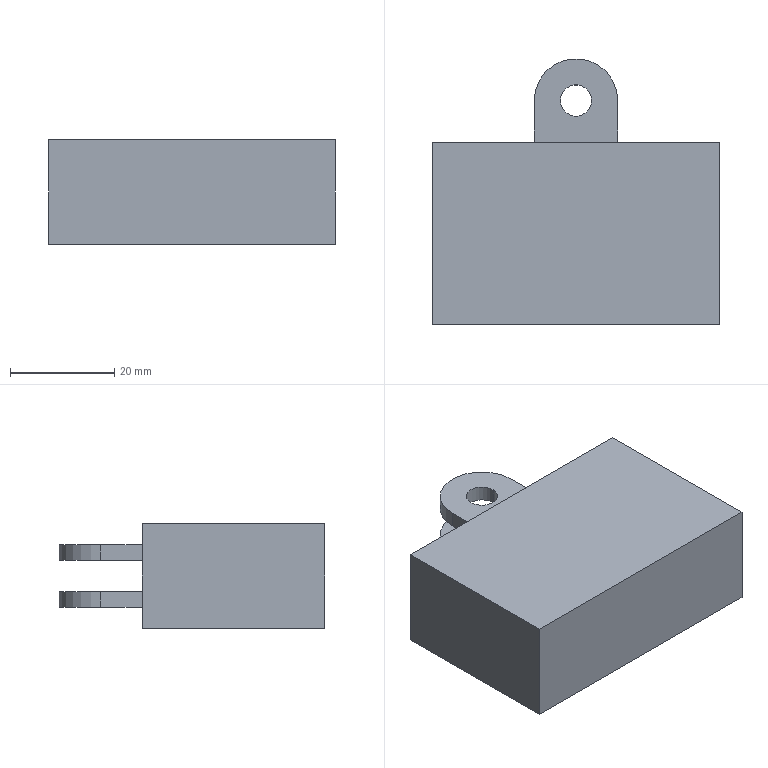Part | SolidWorks | features ICE 3, Extrusion 1 | 1 solid | 20 faces | box 55 x 51 x 20 mm | volume 39702 mm3 | plane 14 | cylinder 6 | commonest cylinder face diameters 6 x4 16 x2
STEP:
#1=CARTESIAN_POINT('',(-3.,25.5,4.));
#2=VERTEX_POINT('',#1);
#3=CARTESIAN_POINT('',(3.,25.5,4.));
#4=VERTEX_POINT('',#3);
#5=CARTESIAN_POINT('',(0.,25.5,4.));
#6=DIRECTION('',(0.,0.,1.));
#7=DIRECTION('',(1.,0.,0.));
#8=AXIS2_PLACEMENT_3D('',#5,#6,#7);
#9=CIRCLE('',#8,3.);
#10=EDGE_CURVE('',#2,#4,#9,.T.);
#11=ORIENTED_EDGE('',*,*,#10,.F.);
#12=CARTESIAN_POINT('',(-3.,25.5,7.));
#13=VERTEX_POINT('',#12);
#14=CARTESIAN_POINT('',(-3.,25.5,0.));
#15=DIRECTION('',(0.,0.,1.));
#16=VECTOR('',#15,1000.);
#17=LINE('',#14,#16);
#18=EDGE_CURVE('',#2,#13,#17,.T.);
#19=ORIENTED_EDGE('',*,*,#18,.T.);
#20=CARTESIAN_POINT('',(3.,25.5,7.));
#21=VERTEX_POINT('',#20);
#22=CARTESIAN_POINT('',(0.,25.5,7.));
#23=DIRECTION('',(0.,0.,1.));
#24=DIRECTION('',(1.,0.,0.));
#25=AXIS2_PLACEMENT_3D('',#22,#23,#24);
#26=CIRCLE('',#25,3.);
#27=EDGE_CURVE('',#13,#21,#26,.T.);
#28=ORIENTED_EDGE('',*,*,#27,.T.);
#29=CARTESIAN_POINT('',(3.,25.5,0.));
#30=DIRECTION('',(0.,0.,1.));
#31=VECTOR('',#30,1000.);
#32=LINE('',#29,#31);
#33=EDGE_CURVE('',#4,#21,#32,.T.);
#34=ORIENTED_EDGE('',*,*,#33,.F.);
#35=EDGE_LOOP('',(#11,#19,#28,#34));
#36=FACE_OUTER_BOUND('',#35,.T.);
#37=CARTESIAN_POINT('',(0.,25.5,0.));
#38=DIRECTION('',(0.,0.,1.));
#39=DIRECTION('',(1.,0.,0.));
#40=AXIS2_PLACEMENT_3D('',#37,#38,#39);
#41=CYLINDRICAL_SURFACE('',#40,3.);
#42=ADVANCED_FACE('',(#36),#41,.F.);
#43=CARTESIAN_POINT('',(3.,25.5,13.));
#44=VERTEX_POINT('',#43);
#45=CARTESIAN_POINT('',(-3.,25.5,13.));
#46=VERTEX_POINT('',#45);
#47=CARTESIAN_POINT('',(0.,25.5,13.));
#48=DIRECTION('',(0.,0.,-1.));
#49=DIRECTION('',(-1.,0.,0.));
#50=AXIS2_PLACEMENT_3D('',#47,#48,#49);
#51=CIRCLE('',#50,3.);
#52=EDGE_CURVE('',#44,#46,#51,.T.);
#53=ORIENTED_EDGE('',*,*,#52,.T.);
#54=CARTESIAN_POINT('',(-3.,25.5,16.));
#55=VERTEX_POINT('',#54);
#56=CARTESIAN_POINT('',(-3.,25.5,0.));
#57=DIRECTION('',(0.,0.,1.));
#58=VECTOR('',#57,1000.);
#59=LINE('',#56,#58);
#60=EDGE_CURVE('',#46,#55,#59,.T.);
#61=ORIENTED_EDGE('',*,*,#60,.T.);
#62=CARTESIAN_POINT('',(3.,25.5,16.));
#63=VERTEX_POINT('',#62);
#64=CARTESIAN_POINT('',(0.,25.5,16.));
#65=DIRECTION('',(0.,0.,1.));
#66=DIRECTION('',(1.,0.,0.));
#67=AXIS2_PLACEMENT_3D('',#64,#65,#66);
#68=CIRCLE('',#67,3.);
#69=EDGE_CURVE('',#55,#63,#68,.T.);
#70=ORIENTED_EDGE('',*,*,#69,.T.);
#71=CARTESIAN_POINT('',(3.,25.5,0.));
#72=DIRECTION('',(0.,0.,1.));
#73=VECTOR('',#72,1000.);
#74=LINE('',#71,#73);
#75=EDGE_CURVE('',#44,#63,#74,.T.);
#76=ORIENTED_EDGE('',*,*,#75,.F.);
#77=EDGE_LOOP('',(#53,#61,#70,#76));
#78=FACE_OUTER_BOUND('',#77,.T.);
#79=CARTESIAN_POINT('',(0.,25.5,0.));
#80=DIRECTION('',(0.,0.,1.));
#81=DIRECTION('',(1.,0.,0.));
#82=AXIS2_PLACEMENT_3D('',#79,#80,#81);
#83=CYLINDRICAL_SURFACE('',#82,3.);
#84=ADVANCED_FACE('',(#78),#83,.F.);
#85=CARTESIAN_POINT('',(-8.,25.5,4.));
#86=VERTEX_POINT('',#85);
#87=CARTESIAN_POINT('',(-8.,17.5,4.));
#88=VERTEX_POINT('',#87);
#89=CARTESIAN_POINT('',(-8.,33.5,4.));
#90=DIRECTION('',(0.,-1.,0.));
#91=VECTOR('',#90,1000.);
#92=LINE('',#89,#91);
#93=EDGE_CURVE('',#86,#88,#92,.T.);
#94=ORIENTED_EDGE('',*,*,#93,.F.);
#95=CARTESIAN_POINT('',(8.,25.5,4.));
#96=VERTEX_POINT('',#95);
#97=CARTESIAN_POINT('',(0.,25.5,4.));
#98=DIRECTION('',(0.,0.,-1.));
#99=DIRECTION('',(1.,0.,0.));
#100=AXIS2_PLACEMENT_3D('',#97,#98,#99);
#101=CIRCLE('',#100,8.);
#102=EDGE_CURVE('',#86,#96,#101,.T.);
#103=ORIENTED_EDGE('',*,*,#102,.T.);
#104=CARTESIAN_POINT('',(8.,17.5,4.));
#105=VERTEX_POINT('',#104);
#106=CARTESIAN_POINT('',(8.,33.5,4.));
#107=DIRECTION('',(0.,-1.,0.));
#108=VECTOR('',#107,1000.);
#109=LINE('',#106,#108);
#110=EDGE_CURVE('',#96,#105,#109,.T.);
#111=ORIENTED_EDGE('',*,*,#110,.T.);
#112=CARTESIAN_POINT('',(-8.,17.5,4.));
#113=DIRECTION('',(-1.,0.,0.));
#114=VECTOR('',#113,1000.);
#115=LINE('',#112,#114);
#116=EDGE_CURVE('',#105,#88,#115,.T.);
#117=ORIENTED_EDGE('',*,*,#116,.T.);
#118=EDGE_LOOP('',(#94,#103,#111,#117));
#119=FACE_OUTER_BOUND('',#118,.T.);
#120=CARTESIAN_POINT('',(0.,25.5,4.));
#121=DIRECTION('',(0.,0.,1.));
#122=DIRECTION('',(1.,0.,0.));
#123=AXIS2_PLACEMENT_3D('',#120,#121,#122);
#124=CIRCLE('',#123,3.);
#125=EDGE_CURVE('',#4,#2,#124,.T.);
#126=ORIENTED_EDGE('',*,*,#125,.T.);
#127=ORIENTED_EDGE('',*,*,#10,.T.);
#128=EDGE_LOOP('',(#126,#127));
#129=FACE_BOUND('',#128,.T.);
#130=CARTESIAN_POINT('',(-8.,33.5,4.));
#131=DIRECTION('',(0.,0.,1.));
#132=DIRECTION('',(1.,0.,0.));
#133=AXIS2_PLACEMENT_3D('',#130,#131,#132);
#134=PLANE('',#133);
#135=ADVANCED_FACE('',(#119,#129),#134,.F.);
#136=CARTESIAN_POINT('',(8.,25.5,16.));
#137=VERTEX_POINT('',#136);
#138=CARTESIAN_POINT('',(8.,17.5,16.));
#139=VERTEX_POINT('',#138);
#140=CARTESIAN_POINT('',(8.,33.5,16.));
#141=DIRECTION('',(0.,-1.,0.));
#142=VECTOR('',#141,1000.);
#143=LINE('',#140,#142);
#144=EDGE_CURVE('',#137,#139,#143,.T.);
#145=ORIENTED_EDGE('',*,*,#144,.F.);
#146=CARTESIAN_POINT('',(-8.,25.5,16.));
#147=VERTEX_POINT('',#146);
#148=CARTESIAN_POINT('',(0.,25.5,16.));
#149=DIRECTION('',(0.,0.,-1.));
#150=DIRECTION('',(1.,0.,0.));
#151=AXIS2_PLACEMENT_3D('',#148,#149,#150);
#152=CIRCLE('',#151,8.);
#153=EDGE_CURVE('',#147,#137,#152,.T.);
#154=ORIENTED_EDGE('',*,*,#153,.F.);
#155=CARTESIAN_POINT('',(-8.,17.5,16.));
#156=VERTEX_POINT('',#155);
#157=CARTESIAN_POINT('',(-8.,33.5,16.));
#158=DIRECTION('',(0.,-1.,0.));
#159=VECTOR('',#158,1000.);
#160=LINE('',#157,#159);
#161=EDGE_CURVE('',#147,#156,#160,.T.);
#162=ORIENTED_EDGE('',*,*,#161,.T.);
#163=CARTESIAN_POINT('',(-8.,17.5,16.));
#164=DIRECTION('',(1.,0.,0.));
#165=VECTOR('',#164,1000.);
#166=LINE('',#163,#165);
#167=EDGE_CURVE('',#156,#139,#166,.T.);
#168=ORIENTED_EDGE('',*,*,#167,.T.);
#169=EDGE_LOOP('',(#145,#154,#162,#168));
#170=FACE_OUTER_BOUND('',#169,.T.);
#171=CARTESIAN_POINT('',(0.,25.5,16.));
#172=DIRECTION('',(0.,0.,1.));
#173=DIRECTION('',(1.,0.,0.));
#174=AXIS2_PLACEMENT_3D('',#171,#172,#173);
#175=CIRCLE('',#174,3.);
#176=EDGE_CURVE('',#63,#55,#175,.T.);
#177=ORIENTED_EDGE('',*,*,#176,.F.);
#178=ORIENTED_EDGE('',*,*,#69,.F.);
#179=EDGE_LOOP('',(#177,#178));
#180=FACE_BOUND('',#179,.T.);
#181=CARTESIAN_POINT('',(-8.,33.5,16.));
#182=DIRECTION('',(0.,0.,-1.));
#183=DIRECTION('',(-1.,0.,0.));
#184=AXIS2_PLACEMENT_3D('',#181,#182,#183);
#185=PLANE('',#184);
#186=ADVANCED_FACE('',(#170,#180),#185,.F.);
#187=CARTESIAN_POINT('',(-8.,25.5,7.));
#188=VERTEX_POINT('',#187);
#189=CARTESIAN_POINT('',(8.,25.5,7.));
#190=VERTEX_POINT('',#189);
#191=CARTESIAN_POINT('',(0.,25.5,7.));
#192=DIRECTION('',(0.,0.,-1.));
#193=DIRECTION('',(1.,0.,0.));
#194=AXIS2_PLACEMENT_3D('',#191,#192,#193);
#195=CIRCLE('',#194,8.);
#196=EDGE_CURVE('',#188,#190,#195,.T.);
#197=ORIENTED_EDGE('',*,*,#196,.F.);
#198=CARTESIAN_POINT('',(-8.,17.5,7.));
#199=VERTEX_POINT('',#198);
#200=CARTESIAN_POINT('',(-8.,33.5,7.));
#201=DIRECTION('',(0.,-1.,0.));
#202=VECTOR('',#201,1000.);
#203=LINE('',#200,#202);
#204=EDGE_CURVE('',#188,#199,#203,.T.);
#205=ORIENTED_EDGE('',*,*,#204,.T.);
#206=CARTESIAN_POINT('',(8.,17.5,7.));
#207=VERTEX_POINT('',#206);
#208=CARTESIAN_POINT('',(-8.,17.5,7.));
#209=DIRECTION('',(-1.,0.,0.));
#210=VECTOR('',#209,1000.);
#211=LINE('',#208,#210);
#212=EDGE_CURVE('',#207,#199,#211,.T.);
#213=ORIENTED_EDGE('',*,*,#212,.F.);
#214=CARTESIAN_POINT('',(8.,33.5,7.));
#215=DIRECTION('',(0.,-1.,0.));
#216=VECTOR('',#215,1000.);
#217=LINE('',#214,#216);
#218=EDGE_CURVE('',#190,#207,#217,.T.);
#219=ORIENTED_EDGE('',*,*,#218,.F.);
#220=EDGE_LOOP('',(#197,#205,#213,#219));
#221=FACE_OUTER_BOUND('',#220,.T.);
#222=CARTESIAN_POINT('',(0.,25.5,7.));
#223=DIRECTION('',(0.,0.,1.));
#224=DIRECTION('',(1.,0.,0.));
#225=AXIS2_PLACEMENT_3D('',#222,#223,#224);
#226=CIRCLE('',#225,3.);
#227=EDGE_CURVE('',#21,#13,#226,.T.);
#228=ORIENTED_EDGE('',*,*,#227,.F.);
#229=ORIENTED_EDGE('',*,*,#27,.F.);
#230=EDGE_LOOP('',(#228,#229));
#231=FACE_BOUND('',#230,.T.);
#232=CARTESIAN_POINT('',(-8.,33.5,7.));
#233=DIRECTION('',(0.,0.,1.));
#234=DIRECTION('',(1.,0.,0.));
#235=AXIS2_PLACEMENT_3D('',#232,#233,#234);
#236=PLANE('',#235);
#237=ADVANCED_FACE('',(#221,#231),#236,.T.);
#238=CARTESIAN_POINT('',(8.,25.5,13.));
#239=VERTEX_POINT('',#238);
#240=CARTESIAN_POINT('',(-8.,25.5,13.));
#241=VERTEX_POINT('',#240);
#242=CARTESIAN_POINT('',(0.,25.5,13.));
#243=DIRECTION('',(0.,0.,1.));
#244=DIRECTION('',(-1.,0.,0.));
#245=AXIS2_PLACEMENT_3D('',#242,#243,#244);
#246=CIRCLE('',#245,8.);
#247=EDGE_CURVE('',#239,#241,#246,.T.);
#248=ORIENTED_EDGE('',*,*,#247,.F.);
#249=CARTESIAN_POINT('',(8.,17.5,13.));
#250=VERTEX_POINT('',#249);
#251=CARTESIAN_POINT('',(8.,33.5,13.));
#252=DIRECTION('',(0.,-1.,0.));
#253=VECTOR('',#252,1000.);
#254=LINE('',#251,#253);
#255=EDGE_CURVE('',#239,#250,#254,.T.);
#256=ORIENTED_EDGE('',*,*,#255,.T.);
#257=CARTESIAN_POINT('',(-8.,17.5,13.));
#258=VERTEX_POINT('',#257);
#259=CARTESIAN_POINT('',(-8.,17.5,13.));
#260=DIRECTION('',(1.,0.,0.));
#261=VECTOR('',#260,1000.);
#262=LINE('',#259,#261);
#263=EDGE_CURVE('',#258,#250,#262,.T.);
#264=ORIENTED_EDGE('',*,*,#263,.F.);
#265=CARTESIAN_POINT('',(-8.,33.5,13.));
#266=DIRECTION('',(0.,-1.,0.));
#267=VECTOR('',#266,1000.);
#268=LINE('',#265,#267);
#269=EDGE_CURVE('',#241,#258,#268,.T.);
#270=ORIENTED_EDGE('',*,*,#269,.F.);
#271=EDGE_LOOP('',(#248,#256,#264,#270));
#272=FACE_OUTER_BOUND('',#271,.T.);
#273=ORIENTED_EDGE('',*,*,#52,.F.);
#274=CARTESIAN_POINT('',(0.,25.5,13.));
#275=DIRECTION('',(0.,0.,-1.));
#276=DIRECTION('',(-1.,0.,0.));
#277=AXIS2_PLACEMENT_3D('',#274,#275,#276);
#278=CIRCLE('',#277,3.);
#279=EDGE_CURVE('',#46,#44,#278,.T.);
#280=ORIENTED_EDGE('',*,*,#279,.F.);
#281=EDGE_LOOP('',(#273,#280));
#282=FACE_BOUND('',#281,.T.);
#283=CARTESIAN_POINT('',(-8.,33.5,13.));
#284=DIRECTION('',(0.,0.,-1.));
#285=DIRECTION('',(-1.,0.,0.));
#286=AXIS2_PLACEMENT_3D('',#283,#284,#285);
#287=PLANE('',#286);
#288=ADVANCED_FACE('',(#272,#282),#287,.T.);
#289=ORIENTED_EDGE('',*,*,#110,.F.);
#290=CARTESIAN_POINT('',(8.,25.5,0.));
#291=DIRECTION('',(0.,0.,1.));
#292=VECTOR('',#291,1000.);
#293=LINE('',#290,#292);
#294=EDGE_CURVE('',#96,#190,#293,.T.);
#295=ORIENTED_EDGE('',*,*,#294,.T.);
#296=ORIENTED_EDGE('',*,*,#218,.T.);
#297=CARTESIAN_POINT('',(8.,17.5,4.));
#298=DIRECTION('',(0.,0.,-1.));
#299=VECTOR('',#298,1000.);
#300=LINE('',#297,#299);
#301=EDGE_CURVE('',#207,#105,#300,.T.);
#302=ORIENTED_EDGE('',*,*,#301,.T.);
#303=EDGE_LOOP('',(#289,#295,#296,#302));
#304=FACE_OUTER_BOUND('',#303,.T.);
#305=CARTESIAN_POINT('',(8.,33.5,4.));
#306=DIRECTION('',(-1.,0.,0.));
#307=DIRECTION('',(0.,0.,1.));
#308=AXIS2_PLACEMENT_3D('',#305,#306,#307);
#309=PLANE('',#308);
#310=ADVANCED_FACE('',(#304),#309,.F.);
#311=ORIENTED_EDGE('',*,*,#255,.F.);
#312=CARTESIAN_POINT('',(8.,25.5,0.));
#313=DIRECTION('',(0.,0.,1.));
#314=VECTOR('',#313,1000.);
#315=LINE('',#312,#314);
#316=EDGE_CURVE('',#239,#137,#315,.T.);
#317=ORIENTED_EDGE('',*,*,#316,.T.);
#318=ORIENTED_EDGE('',*,*,#144,.T.);
#319=CARTESIAN_POINT('',(8.,17.5,4.));
#320=DIRECTION('',(0.,0.,-1.));
#321=VECTOR('',#320,1000.);
#322=LINE('',#319,#321);
#323=EDGE_CURVE('',#139,#250,#322,.T.);
#324=ORIENTED_EDGE('',*,*,#323,.T.);
#325=EDGE_LOOP('',(#311,#317,#318,#324));
#326=FACE_OUTER_BOUND('',#325,.T.);
#327=CARTESIAN_POINT('',(8.,33.5,4.));
#328=DIRECTION('',(-1.,0.,0.));
#329=DIRECTION('',(0.,0.,1.));
#330=AXIS2_PLACEMENT_3D('',#327,#328,#329);
#331=PLANE('',#330);
#332=ADVANCED_FACE('',(#326),#331,.F.);
#333=ORIENTED_EDGE('',*,*,#204,.F.);
#334=CARTESIAN_POINT('',(-8.,25.5,0.));
#335=DIRECTION('',(0.,0.,1.));
#336=VECTOR('',#335,1000.);
#337=LINE('',#334,#336);
#338=EDGE_CURVE('',#86,#188,#337,.T.);
#339=ORIENTED_EDGE('',*,*,#338,.F.);
#340=ORIENTED_EDGE('',*,*,#93,.T.);
#341=CARTESIAN_POINT('',(-8.,17.5,4.));
#342=DIRECTION('',(0.,0.,1.));
#343=VECTOR('',#342,1000.);
#344=LINE('',#341,#343);
#345=EDGE_CURVE('',#88,#199,#344,.T.);
#346=ORIENTED_EDGE('',*,*,#345,.T.);
#347=EDGE_LOOP('',(#333,#339,#340,#346));
#348=FACE_OUTER_BOUND('',#347,.T.);
#349=CARTESIAN_POINT('',(-8.,33.5,4.));
#350=DIRECTION('',(1.,0.,0.));
#351=DIRECTION('',(0.,0.,-1.));
#352=AXIS2_PLACEMENT_3D('',#349,#350,#351);
#353=PLANE('',#352);
#354=ADVANCED_FACE('',(#348),#353,.F.);
#355=ORIENTED_EDGE('',*,*,#161,.F.);
#356=CARTESIAN_POINT('',(-8.,25.5,0.));
#357=DIRECTION('',(0.,0.,1.));
#358=VECTOR('',#357,1000.);
#359=LINE('',#356,#358);
#360=EDGE_CURVE('',#241,#147,#359,.T.);
#361=ORIENTED_EDGE('',*,*,#360,.F.);
#362=ORIENTED_EDGE('',*,*,#269,.T.);
#363=CARTESIAN_POINT('',(-8.,17.5,4.));
#364=DIRECTION('',(0.,0.,1.));
#365=VECTOR('',#364,1000.);
#366=LINE('',#363,#365);
#367=EDGE_CURVE('',#258,#156,#366,.T.);
#368=ORIENTED_EDGE('',*,*,#367,.T.);
#369=EDGE_LOOP('',(#355,#361,#362,#368));
#370=FACE_OUTER_BOUND('',#369,.T.);
#371=CARTESIAN_POINT('',(-8.,33.5,4.));
#372=DIRECTION('',(1.,0.,0.));
#373=DIRECTION('',(0.,0.,-1.));
#374=AXIS2_PLACEMENT_3D('',#371,#372,#373);
#375=PLANE('',#374);
#376=ADVANCED_FACE('',(#370),#375,.F.);
#377=ORIENTED_EDGE('',*,*,#301,.F.);
#378=ORIENTED_EDGE('',*,*,#212,.T.);
#379=ORIENTED_EDGE('',*,*,#345,.F.);
#380=ORIENTED_EDGE('',*,*,#116,.F.);
#381=EDGE_LOOP('',(#377,#378,#379,#380));
#382=FACE_BOUND('',#381,.T.);
#383=CARTESIAN_POINT('',(27.5,17.5,0.));
#384=VERTEX_POINT('',#383);
#385=CARTESIAN_POINT('',(-27.5,17.5,0.));
#386=VERTEX_POINT('',#385);
#387=CARTESIAN_POINT('',(-27.5,17.5,0.));
#388=DIRECTION('',(-1.,0.,0.));
#389=VECTOR('',#388,1000.);
#390=LINE('',#387,#389);
#391=EDGE_CURVE('',#384,#386,#390,.T.);
#392=ORIENTED_EDGE('',*,*,#391,.T.);
#393=CARTESIAN_POINT('',(-27.5,17.5,20.));
#394=VERTEX_POINT('',#393);
#395=CARTESIAN_POINT('',(-27.5,17.5,20.));
#396=DIRECTION('',(0.,0.,-1.));
#397=VECTOR('',#396,1000.);
#398=LINE('',#395,#397);
#399=EDGE_CURVE('',#394,#386,#398,.T.);
#400=ORIENTED_EDGE('',*,*,#399,.F.);
#401=CARTESIAN_POINT('',(27.5,17.5,20.));
#402=VERTEX_POINT('',#401);
#403=CARTESIAN_POINT('',(-27.5,17.5,20.));
#404=DIRECTION('',(-1.,0.,0.));
#405=VECTOR('',#404,1000.);
#406=LINE('',#403,#405);
#407=EDGE_CURVE('',#402,#394,#406,.T.);
#408=ORIENTED_EDGE('',*,*,#407,.F.);
#409=CARTESIAN_POINT('',(27.5,17.5,20.));
#410=DIRECTION('',(0.,0.,-1.));
#411=VECTOR('',#410,1000.);
#412=LINE('',#409,#411);
#413=EDGE_CURVE('',#402,#384,#412,.T.);
#414=ORIENTED_EDGE('',*,*,#413,.T.);
#415=EDGE_LOOP('',(#392,#400,#408,#414));
#416=FACE_OUTER_BOUND('',#415,.T.);
#417=ORIENTED_EDGE('',*,*,#323,.F.);
#418=ORIENTED_EDGE('',*,*,#167,.F.);
#419=ORIENTED_EDGE('',*,*,#367,.F.);
#420=ORIENTED_EDGE('',*,*,#263,.T.);
#421=EDGE_LOOP('',(#417,#418,#419,#420));
#422=FACE_BOUND('',#421,.T.);
#423=CARTESIAN_POINT('',(-27.5,17.5,20.));
#424=DIRECTION('',(0.,-1.,0.));
#425=DIRECTION('',(0.,0.,-1.));
#426=AXIS2_PLACEMENT_3D('',#423,#424,#425);
#427=PLANE('',#426);
#428=ADVANCED_FACE('',(#382,#416,#422),#427,.F.);
#429=CARTESIAN_POINT('',(27.5,-17.5,0.));
#430=VERTEX_POINT('',#429);
#431=CARTESIAN_POINT('',(27.5,17.5,0.));
#432=DIRECTION('',(0.,1.,0.));
#433=VECTOR('',#432,1000.);
#434=LINE('',#431,#433);
#435=EDGE_CURVE('',#430,#384,#434,.T.);
#436=ORIENTED_EDGE('',*,*,#435,.T.);
#437=ORIENTED_EDGE('',*,*,#413,.F.);
#438=CARTESIAN_POINT('',(27.5,-17.5,20.));
#439=VERTEX_POINT('',#438);
#440=CARTESIAN_POINT('',(27.5,17.5,20.));
#441=DIRECTION('',(0.,1.,0.));
#442=VECTOR('',#441,1000.);
#443=LINE('',#440,#442);
#444=EDGE_CURVE('',#439,#402,#443,.T.);
#445=ORIENTED_EDGE('',*,*,#444,.F.);
#446=CARTESIAN_POINT('',(27.5,-17.5,20.));
#447=DIRECTION('',(0.,0.,-1.));
#448=VECTOR('',#447,1000.);
#449=LINE('',#446,#448);
#450=EDGE_CURVE('',#439,#430,#449,.T.);
#451=ORIENTED_EDGE('',*,*,#450,.T.);
#452=EDGE_LOOP('',(#436,#437,#445,#451));
#453=FACE_OUTER_BOUND('',#452,.T.);
#454=CARTESIAN_POINT('',(27.5,17.5,20.));
#455=DIRECTION('',(-1.,0.,0.));
#456=DIRECTION('',(0.,-1.,0.));
#457=AXIS2_PLACEMENT_3D('',#454,#455,#456);
#458=PLANE('',#457);
#459=ADVANCED_FACE('',(#453),#458,.F.);
#460=CARTESIAN_POINT('',(-27.5,-17.5,0.));
#461=VERTEX_POINT('',#460);
#462=CARTESIAN_POINT('',(-27.5,17.5,0.));
#463=DIRECTION('',(0.,-1.,0.));
#464=VECTOR('',#463,1000.);
#465=LINE('',#462,#464);
#466=EDGE_CURVE('',#386,#461,#465,.T.);
#467=ORIENTED_EDGE('',*,*,#466,.T.);
#468=CARTESIAN_POINT('',(-27.5,-17.5,20.));
#469=VERTEX_POINT('',#468);
#470=CARTESIAN_POINT('',(-27.5,-17.5,20.));
#471=DIRECTION('',(0.,0.,-1.));
#472=VECTOR('',#471,1000.);
#473=LINE('',#470,#472);
#474=EDGE_CURVE('',#469,#461,#473,.T.);
#475=ORIENTED_EDGE('',*,*,#474,.F.);
#476=CARTESIAN_POINT('',(-27.5,17.5,20.));
#477=DIRECTION('',(0.,-1.,0.));
#478=VECTOR('',#477,1000.);
#479=LINE('',#476,#478);
#480=EDGE_CURVE('',#394,#469,#479,.T.);
#481=ORIENTED_EDGE('',*,*,#480,.F.);
#482=ORIENTED_EDGE('',*,*,#399,.T.);
#483=EDGE_LOOP('',(#467,#475,#481,#482));
#484=FACE_OUTER_BOUND('',#483,.T.);
#485=CARTESIAN_POINT('',(-27.5,17.5,20.));
#486=DIRECTION('',(1.,0.,0.));
#487=DIRECTION('',(0.,1.,0.));
#488=AXIS2_PLACEMENT_3D('',#485,#486,#487);
#489=PLANE('',#488);
#490=ADVANCED_FACE('',(#484),#489,.F.);
#491=CARTESIAN_POINT('',(-27.5,-17.5,0.));
#492=DIRECTION('',(1.,0.,0.));
#493=VECTOR('',#492,1000.);
#494=LINE('',#491,#493);
#495=EDGE_CURVE('',#461,#430,#494,.T.);
#496=ORIENTED_EDGE('',*,*,#495,.T.);
#497=ORIENTED_EDGE('',*,*,#450,.F.);
#498=CARTESIAN_POINT('',(-27.5,-17.5,20.));
#499=DIRECTION('',(1.,0.,0.));
#500=VECTOR('',#499,1000.);
#501=LINE('',#498,#500);
#502=EDGE_CURVE('',#469,#439,#501,.T.);
#503=ORIENTED_EDGE('',*,*,#502,.F.);
#504=ORIENTED_EDGE('',*,*,#474,.T.);
#505=EDGE_LOOP('',(#496,#497,#503,#504));
#506=FACE_OUTER_BOUND('',#505,.T.);
#507=CARTESIAN_POINT('',(-27.5,-17.5,20.));
#508=DIRECTION('',(0.,1.,0.));
#509=DIRECTION('',(0.,0.,1.));
#510=AXIS2_PLACEMENT_3D('',#507,#508,#509);
#511=PLANE('',#510);
#512=ADVANCED_FACE('',(#506),#511,.F.);
#513=ORIENTED_EDGE('',*,*,#444,.T.);
#514=ORIENTED_EDGE('',*,*,#407,.T.);
#515=ORIENTED_EDGE('',*,*,#480,.T.);
#516=ORIENTED_EDGE('',*,*,#502,.T.);
#517=EDGE_LOOP('',(#513,#514,#515,#516));
#518=FACE_OUTER_BOUND('',#517,.T.);
#519=CARTESIAN_POINT('',(0.,0.,20.));
#520=DIRECTION('',(0.,0.,1.));
#521=DIRECTION('',(1.,0.,0.));
#522=AXIS2_PLACEMENT_3D('',#519,#520,#521);
#523=PLANE('',#522);
#524=ADVANCED_FACE('',(#518),#523,.T.);
#525=ORIENTED_EDGE('',*,*,#435,.F.);
#526=ORIENTED_EDGE('',*,*,#495,.F.);
#527=ORIENTED_EDGE('',*,*,#466,.F.);
#528=ORIENTED_EDGE('',*,*,#391,.F.);
#529=EDGE_LOOP('',(#525,#526,#527,#528));
#530=FACE_OUTER_BOUND('',#529,.T.);
#531=CARTESIAN_POINT('',(0.,0.,0.));
#532=DIRECTION('',(0.,0.,1.));
#533=DIRECTION('',(1.,0.,0.));
#534=AXIS2_PLACEMENT_3D('',#531,#532,#533);
#535=PLANE('',#534);
#536=ADVANCED_FACE('',(#530),#535,.F.);
#537=ORIENTED_EDGE('',*,*,#153,.T.);
#538=ORIENTED_EDGE('',*,*,#316,.F.);
#539=ORIENTED_EDGE('',*,*,#247,.T.);
#540=ORIENTED_EDGE('',*,*,#360,.T.);
#541=EDGE_LOOP('',(#537,#538,#539,#540));
#542=FACE_OUTER_BOUND('',#541,.T.);
#543=CARTESIAN_POINT('',(0.,25.5,0.));
#544=DIRECTION('',(0.,0.,1.));
#545=DIRECTION('',(1.,0.,0.));
#546=AXIS2_PLACEMENT_3D('',#543,#544,#545);
#547=CYLINDRICAL_SURFACE('',#546,8.);
#548=ADVANCED_FACE('',(#542),#547,.T.);
#549=ORIENTED_EDGE('',*,*,#60,.F.);
#550=ORIENTED_EDGE('',*,*,#279,.T.);
#551=ORIENTED_EDGE('',*,*,#75,.T.);
#552=ORIENTED_EDGE('',*,*,#176,.T.);
#553=EDGE_LOOP('',(#549,#550,#551,#552));
#554=FACE_OUTER_BOUND('',#553,.T.);
#555=CARTESIAN_POINT('',(0.,25.5,0.));
#556=DIRECTION('',(0.,0.,1.));
#557=DIRECTION('',(1.,0.,0.));
#558=AXIS2_PLACEMENT_3D('',#555,#556,#557);
#559=CYLINDRICAL_SURFACE('',#558,3.);
#560=ADVANCED_FACE('',(#554),#559,.F.);
#561=ORIENTED_EDGE('',*,*,#196,.T.);
#562=ORIENTED_EDGE('',*,*,#294,.F.);
#563=ORIENTED_EDGE('',*,*,#102,.F.);
#564=ORIENTED_EDGE('',*,*,#338,.T.);
#565=EDGE_LOOP('',(#561,#562,#563,#564));
#566=FACE_OUTER_BOUND('',#565,.T.);
#567=CARTESIAN_POINT('',(0.,25.5,0.));
#568=DIRECTION('',(0.,0.,1.));
#569=DIRECTION('',(1.,0.,0.));
#570=AXIS2_PLACEMENT_3D('',#567,#568,#569);
#571=CYLINDRICAL_SURFACE('',#570,8.);
#572=ADVANCED_FACE('',(#566),#571,.T.);
#573=ORIENTED_EDGE('',*,*,#18,.F.);
#574=ORIENTED_EDGE('',*,*,#125,.F.);
#575=ORIENTED_EDGE('',*,*,#33,.T.);
#576=ORIENTED_EDGE('',*,*,#227,.T.);
#577=EDGE_LOOP('',(#573,#574,#575,#576));
#578=FACE_OUTER_BOUND('',#577,.T.);
#579=CARTESIAN_POINT('',(0.,25.5,0.));
#580=DIRECTION('',(0.,0.,1.));
#581=DIRECTION('',(1.,0.,0.));
#582=AXIS2_PLACEMENT_3D('',#579,#580,#581);
#583=CYLINDRICAL_SURFACE('',#582,3.);
#584=ADVANCED_FACE('',(#578),#583,.F.);
#585=CLOSED_SHELL('',(#42,#84,#135,#186,#237,#288,#310,#332,#354,#376,#428,#459,#490,#512,#524,#536,#548,#560,#572,#584));
#586=MANIFOLD_SOLID_BREP('',#585);
#587=CARTESIAN_POINT('',(0.,0.,0.));
#588=DIRECTION('',(0.,0.,1.));
#589=DIRECTION('',(1.,0.,0.));
#590=AXIS2_PLACEMENT_3D('',#587,#588,#589);
#591=(LENGTH_UNIT()NAMED_UNIT(*)SI_UNIT(.MILLI.,.METRE.));
#592=UNCERTAINTY_MEASURE_WITH_UNIT(LENGTH_MEASURE(0.00001),#591,'','');
#593=(NAMED_UNIT(*)PLANE_ANGLE_UNIT()SI_UNIT($,.RADIAN.));
#594=(NAMED_UNIT(*)SI_UNIT($,.STERADIAN.)SOLID_ANGLE_UNIT());
#595=(GEOMETRIC_REPRESENTATION_CONTEXT(3)GLOBAL_UNCERTAINTY_ASSIGNED_CONTEXT((#592))GLOBAL_UNIT_ASSIGNED_CONTEXT((#591,#593,#594))REPRESENTATION_CONTEXT('',''));
#596=ADVANCED_BREP_SHAPE_REPRESENTATION('',(#586,#590),#595);